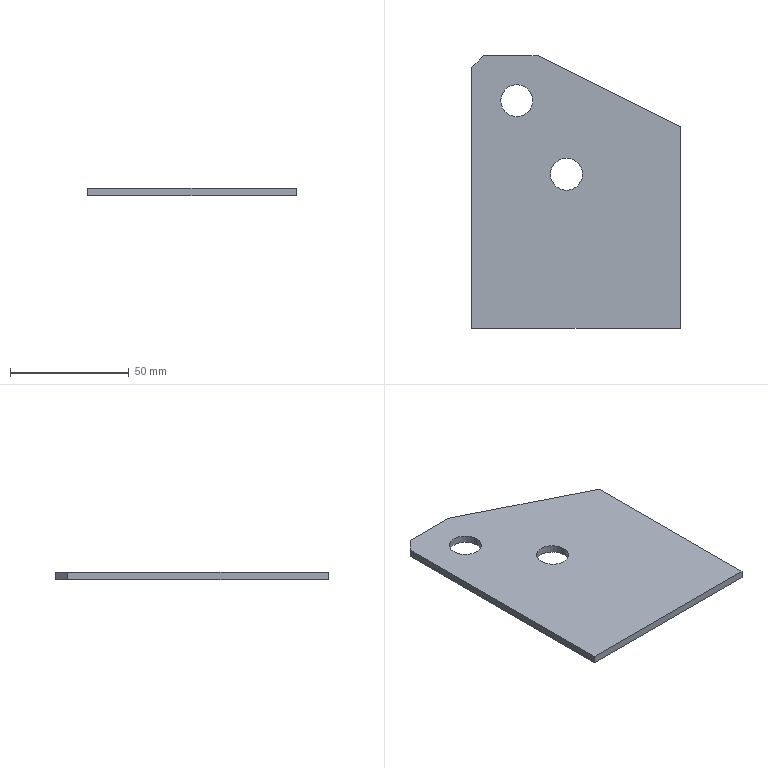Part | SolidWorks | features FlatPattern 1, SMBaseFlange 1, SheetMetal 1 | 1 solid | 12 faces | box 88 x 115 x 3.2 mm | volume 28548 mm3 | plane 8 | cylinder 4 | commonest cylinder face diameters 13.5 x4
STEP:
#1=CARTESIAN_POINT('',(17076.068,-96501.175,-3.2));
#2=VERTEX_POINT('',#1);
#3=CARTESIAN_POINT('',(17089.568,-96501.175,-3.2));
#4=VERTEX_POINT('',#3);
#5=CARTESIAN_POINT('',(17082.818,-96501.175,-3.2));
#6=DIRECTION('',(0.,0.,1.));
#7=DIRECTION('',(1.,0.,0.));
#8=AXIS2_PLACEMENT_3D('',#5,#6,#7);
#9=CIRCLE('',#8,6.75);
#10=EDGE_CURVE('',#2,#4,#9,.T.);
#11=ORIENTED_EDGE('',*,*,#10,.F.);
#12=CARTESIAN_POINT('',(17076.068,-96501.175,0.));
#13=VERTEX_POINT('',#12);
#14=CARTESIAN_POINT('',(17076.068,-96501.175,-3.2));
#15=DIRECTION('',(0.,0.,1.));
#16=VECTOR('',#15,1000.);
#17=LINE('',#14,#16);
#18=EDGE_CURVE('',#2,#13,#17,.T.);
#19=ORIENTED_EDGE('',*,*,#18,.T.);
#20=CARTESIAN_POINT('',(17089.568,-96501.175,0.));
#21=VERTEX_POINT('',#20);
#22=CARTESIAN_POINT('',(17082.818,-96501.175,0.));
#23=DIRECTION('',(0.,0.,1.));
#24=DIRECTION('',(1.,0.,0.));
#25=AXIS2_PLACEMENT_3D('',#22,#23,#24);
#26=CIRCLE('',#25,6.75);
#27=EDGE_CURVE('',#13,#21,#26,.T.);
#28=ORIENTED_EDGE('',*,*,#27,.T.);
#29=CARTESIAN_POINT('',(17089.568,-96501.175,-3.2));
#30=DIRECTION('',(0.,0.,1.));
#31=VECTOR('',#30,1000.);
#32=LINE('',#29,#31);
#33=EDGE_CURVE('',#4,#21,#32,.T.);
#34=ORIENTED_EDGE('',*,*,#33,.F.);
#35=EDGE_LOOP('',(#11,#19,#28,#34));
#36=FACE_OUTER_BOUND('',#35,.T.);
#37=CARTESIAN_POINT('',(17082.818,-96501.175,-3.2));
#38=DIRECTION('',(0.,0.,1.));
#39=DIRECTION('',(1.,0.,0.));
#40=AXIS2_PLACEMENT_3D('',#37,#38,#39);
#41=CYLINDRICAL_SURFACE('',#40,6.75);
#42=ADVANCED_FACE('',(#36),#41,.F.);
#43=CARTESIAN_POINT('',(17097.068,-96532.175,-3.2));
#44=VERTEX_POINT('',#43);
#45=CARTESIAN_POINT('',(17110.568,-96532.175,-3.2));
#46=VERTEX_POINT('',#45);
#47=CARTESIAN_POINT('',(17103.818,-96532.175,-3.2));
#48=DIRECTION('',(0.,0.,1.));
#49=DIRECTION('',(1.,0.,0.));
#50=AXIS2_PLACEMENT_3D('',#47,#48,#49);
#51=CIRCLE('',#50,6.75);
#52=EDGE_CURVE('',#44,#46,#51,.T.);
#53=ORIENTED_EDGE('',*,*,#52,.F.);
#54=CARTESIAN_POINT('',(17097.068,-96532.175,0.));
#55=VERTEX_POINT('',#54);
#56=CARTESIAN_POINT('',(17097.068,-96532.175,-3.2));
#57=DIRECTION('',(0.,0.,1.));
#58=VECTOR('',#57,1000.);
#59=LINE('',#56,#58);
#60=EDGE_CURVE('',#44,#55,#59,.T.);
#61=ORIENTED_EDGE('',*,*,#60,.T.);
#62=CARTESIAN_POINT('',(17110.568,-96532.175,0.));
#63=VERTEX_POINT('',#62);
#64=CARTESIAN_POINT('',(17103.818,-96532.175,0.));
#65=DIRECTION('',(0.,0.,1.));
#66=DIRECTION('',(1.,0.,0.));
#67=AXIS2_PLACEMENT_3D('',#64,#65,#66);
#68=CIRCLE('',#67,6.75);
#69=EDGE_CURVE('',#55,#63,#68,.T.);
#70=ORIENTED_EDGE('',*,*,#69,.T.);
#71=CARTESIAN_POINT('',(17110.568,-96532.175,-3.2));
#72=DIRECTION('',(0.,0.,1.));
#73=VECTOR('',#72,1000.);
#74=LINE('',#71,#73);
#75=EDGE_CURVE('',#46,#63,#74,.T.);
#76=ORIENTED_EDGE('',*,*,#75,.F.);
#77=EDGE_LOOP('',(#53,#61,#70,#76));
#78=FACE_OUTER_BOUND('',#77,.T.);
#79=CARTESIAN_POINT('',(17103.818,-96532.175,-3.2));
#80=DIRECTION('',(0.,0.,1.));
#81=DIRECTION('',(1.,0.,0.));
#82=AXIS2_PLACEMENT_3D('',#79,#80,#81);
#83=CYLINDRICAL_SURFACE('',#82,6.75);
#84=ADVANCED_FACE('',(#78),#83,.F.);
#85=CARTESIAN_POINT('',(17063.818,-96597.175,0.));
#86=VERTEX_POINT('',#85);
#87=CARTESIAN_POINT('',(17151.818,-96597.175,0.));
#88=VERTEX_POINT('',#87);
#89=CARTESIAN_POINT('',(17151.818,-96597.175,0.));
#90=DIRECTION('',(1.,0.,0.));
#91=VECTOR('',#90,1000.);
#92=LINE('',#89,#91);
#93=EDGE_CURVE('',#86,#88,#92,.T.);
#94=ORIENTED_EDGE('',*,*,#93,.F.);
#95=CARTESIAN_POINT('',(17063.818,-96597.175,-3.2));
#96=VERTEX_POINT('',#95);
#97=CARTESIAN_POINT('',(17063.818,-96597.175,-3.2));
#98=DIRECTION('',(0.,0.,1.));
#99=VECTOR('',#98,1000.);
#100=LINE('',#97,#99);
#101=EDGE_CURVE('',#96,#86,#100,.T.);
#102=ORIENTED_EDGE('',*,*,#101,.F.);
#103=CARTESIAN_POINT('',(17151.818,-96597.175,-3.2));
#104=VERTEX_POINT('',#103);
#105=CARTESIAN_POINT('',(17151.818,-96597.175,-3.2));
#106=DIRECTION('',(1.,0.,0.));
#107=VECTOR('',#106,1000.);
#108=LINE('',#105,#107);
#109=EDGE_CURVE('',#96,#104,#108,.T.);
#110=ORIENTED_EDGE('',*,*,#109,.T.);
#111=CARTESIAN_POINT('',(17151.818,-96597.175,-3.2));
#112=DIRECTION('',(0.,0.,1.));
#113=VECTOR('',#112,1000.);
#114=LINE('',#111,#113);
#115=EDGE_CURVE('',#104,#88,#114,.T.);
#116=ORIENTED_EDGE('',*,*,#115,.T.);
#117=EDGE_LOOP('',(#94,#102,#110,#116));
#118=FACE_OUTER_BOUND('',#117,.T.);
#119=CARTESIAN_POINT('',(17151.818,-96597.175,-3.2));
#120=DIRECTION('',(0.,-1.,0.));
#121=DIRECTION('',(0.,0.,-1.));
#122=AXIS2_PLACEMENT_3D('',#119,#120,#121);
#123=PLANE('',#122);
#124=ADVANCED_FACE('',(#118),#123,.T.);
#125=CARTESIAN_POINT('',(17063.818,-96487.175,0.));
#126=VERTEX_POINT('',#125);
#127=CARTESIAN_POINT('',(17063.818,-96597.175,0.));
#128=DIRECTION('',(0.,-1.,0.));
#129=VECTOR('',#128,1000.);
#130=LINE('',#127,#129);
#131=EDGE_CURVE('',#126,#86,#130,.T.);
#132=ORIENTED_EDGE('',*,*,#131,.F.);
#133=CARTESIAN_POINT('',(17063.818,-96487.175,-3.2));
#134=VERTEX_POINT('',#133);
#135=CARTESIAN_POINT('',(17063.818,-96487.175,-3.2));
#136=DIRECTION('',(0.,0.,1.));
#137=VECTOR('',#136,1000.);
#138=LINE('',#135,#137);
#139=EDGE_CURVE('',#134,#126,#138,.T.);
#140=ORIENTED_EDGE('',*,*,#139,.F.);
#141=CARTESIAN_POINT('',(17063.818,-96584.675,-3.2));
#142=DIRECTION('',(0.,-1.,0.));
#143=VECTOR('',#142,1000.);
#144=LINE('',#141,#143);
#145=EDGE_CURVE('',#134,#96,#144,.T.);
#146=ORIENTED_EDGE('',*,*,#145,.T.);
#147=ORIENTED_EDGE('',*,*,#101,.T.);
#148=EDGE_LOOP('',(#132,#140,#146,#147));
#149=FACE_OUTER_BOUND('',#148,.T.);
#150=CARTESIAN_POINT('',(17063.818,-96597.175,-3.2));
#151=DIRECTION('',(-1.,0.,0.));
#152=DIRECTION('',(0.,0.,1.));
#153=AXIS2_PLACEMENT_3D('',#150,#151,#152);
#154=PLANE('',#153);
#155=ADVANCED_FACE('',(#149),#154,.T.);
#156=CARTESIAN_POINT('',(17068.818,-96482.175,0.));
#157=VERTEX_POINT('',#156);
#158=CARTESIAN_POINT('',(17068.818,-96482.175,0.));
#159=DIRECTION('',(-0.7071,-0.7071,0.));
#160=VECTOR('',#159,1000.);
#161=LINE('',#158,#160);
#162=EDGE_CURVE('',#157,#126,#161,.T.);
#163=ORIENTED_EDGE('',*,*,#162,.F.);
#164=CARTESIAN_POINT('',(17068.818,-96482.175,-3.2));
#165=VERTEX_POINT('',#164);
#166=CARTESIAN_POINT('',(17068.818,-96482.175,-3.2));
#167=DIRECTION('',(0.,0.,1.));
#168=VECTOR('',#167,1000.);
#169=LINE('',#166,#168);
#170=EDGE_CURVE('',#165,#157,#169,.T.);
#171=ORIENTED_EDGE('',*,*,#170,.F.);
#172=CARTESIAN_POINT('',(17068.818,-96482.175,-3.2));
#173=DIRECTION('',(-0.7071,-0.7071,0.));
#174=VECTOR('',#173,1000.);
#175=LINE('',#172,#174);
#176=EDGE_CURVE('',#165,#134,#175,.T.);
#177=ORIENTED_EDGE('',*,*,#176,.T.);
#178=ORIENTED_EDGE('',*,*,#139,.T.);
#179=EDGE_LOOP('',(#163,#171,#177,#178));
#180=FACE_OUTER_BOUND('',#179,.T.);
#181=CARTESIAN_POINT('',(17068.818,-96482.175,-3.2));
#182=DIRECTION('',(-0.7071,0.7071,0.));
#183=DIRECTION('',(-0.7071,-0.7071,0.));
#184=AXIS2_PLACEMENT_3D('',#181,#182,#183);
#185=PLANE('',#184);
#186=ADVANCED_FACE('',(#180),#185,.T.);
#187=CARTESIAN_POINT('',(17091.818,-96482.175,0.));
#188=VERTEX_POINT('',#187);
#189=CARTESIAN_POINT('',(17068.818,-96482.175,0.));
#190=DIRECTION('',(-1.,0.,0.));
#191=VECTOR('',#190,1000.);
#192=LINE('',#189,#191);
#193=EDGE_CURVE('',#188,#157,#192,.T.);
#194=ORIENTED_EDGE('',*,*,#193,.F.);
#195=CARTESIAN_POINT('',(17091.818,-96482.175,-3.2));
#196=VERTEX_POINT('',#195);
#197=CARTESIAN_POINT('',(17091.818,-96482.175,-3.2));
#198=DIRECTION('',(0.,0.,1.));
#199=VECTOR('',#198,1000.);
#200=LINE('',#197,#199);
#201=EDGE_CURVE('',#196,#188,#200,.T.);
#202=ORIENTED_EDGE('',*,*,#201,.F.);
#203=CARTESIAN_POINT('',(17068.818,-96482.175,-3.2));
#204=DIRECTION('',(-1.,0.,0.));
#205=VECTOR('',#204,1000.);
#206=LINE('',#203,#205);
#207=EDGE_CURVE('',#196,#165,#206,.T.);
#208=ORIENTED_EDGE('',*,*,#207,.T.);
#209=ORIENTED_EDGE('',*,*,#170,.T.);
#210=EDGE_LOOP('',(#194,#202,#208,#209));
#211=FACE_OUTER_BOUND('',#210,.T.);
#212=CARTESIAN_POINT('',(17068.818,-96482.175,-3.2));
#213=DIRECTION('',(0.,1.,0.));
#214=DIRECTION('',(0.,0.,1.));
#215=AXIS2_PLACEMENT_3D('',#212,#213,#214);
#216=PLANE('',#215);
#217=ADVANCED_FACE('',(#211),#216,.T.);
#218=CARTESIAN_POINT('',(17151.818,-96512.175,0.));
#219=VERTEX_POINT('',#218);
#220=CARTESIAN_POINT('',(17091.818,-96482.175,0.));
#221=DIRECTION('',(-0.8944,0.4472,0.));
#222=VECTOR('',#221,1000.);
#223=LINE('',#220,#222);
#224=EDGE_CURVE('',#219,#188,#223,.T.);
#225=ORIENTED_EDGE('',*,*,#224,.F.);
#226=CARTESIAN_POINT('',(17151.818,-96512.175,-3.2));
#227=VERTEX_POINT('',#226);
#228=CARTESIAN_POINT('',(17151.818,-96512.175,-3.2));
#229=DIRECTION('',(0.,0.,1.));
#230=VECTOR('',#229,1000.);
#231=LINE('',#228,#230);
#232=EDGE_CURVE('',#227,#219,#231,.T.);
#233=ORIENTED_EDGE('',*,*,#232,.F.);
#234=CARTESIAN_POINT('',(17091.818,-96482.175,-3.2));
#235=DIRECTION('',(-0.8944,0.4472,0.));
#236=VECTOR('',#235,1000.);
#237=LINE('',#234,#236);
#238=EDGE_CURVE('',#227,#196,#237,.T.);
#239=ORIENTED_EDGE('',*,*,#238,.T.);
#240=ORIENTED_EDGE('',*,*,#201,.T.);
#241=EDGE_LOOP('',(#225,#233,#239,#240));
#242=FACE_OUTER_BOUND('',#241,.T.);
#243=CARTESIAN_POINT('',(17091.818,-96482.175,-3.2));
#244=DIRECTION('',(0.4472,0.8944,0.));
#245=DIRECTION('',(-0.8944,0.4472,0.));
#246=AXIS2_PLACEMENT_3D('',#243,#244,#245);
#247=PLANE('',#246);
#248=ADVANCED_FACE('',(#242),#247,.T.);
#249=CARTESIAN_POINT('',(17151.818,-96512.175,0.));
#250=DIRECTION('',(0.,1.,0.));
#251=VECTOR('',#250,1000.);
#252=LINE('',#249,#251);
#253=EDGE_CURVE('',#88,#219,#252,.T.);
#254=ORIENTED_EDGE('',*,*,#253,.F.);
#255=ORIENTED_EDGE('',*,*,#115,.F.);
#256=CARTESIAN_POINT('',(17151.818,-96584.675,-3.2));
#257=DIRECTION('',(0.,1.,0.));
#258=VECTOR('',#257,1000.);
#259=LINE('',#256,#258);
#260=EDGE_CURVE('',#104,#227,#259,.T.);
#261=ORIENTED_EDGE('',*,*,#260,.T.);
#262=ORIENTED_EDGE('',*,*,#232,.T.);
#263=EDGE_LOOP('',(#254,#255,#261,#262));
#264=FACE_OUTER_BOUND('',#263,.T.);
#265=CARTESIAN_POINT('',(17151.818,-96512.175,-3.2));
#266=DIRECTION('',(1.,0.,0.));
#267=DIRECTION('',(0.,0.,-1.));
#268=AXIS2_PLACEMENT_3D('',#265,#266,#267);
#269=PLANE('',#268);
#270=ADVANCED_FACE('',(#264),#269,.T.);
#271=CARTESIAN_POINT('',(17082.818,-96501.175,-3.2));
#272=DIRECTION('',(0.,0.,1.));
#273=DIRECTION('',(1.,0.,0.));
#274=AXIS2_PLACEMENT_3D('',#271,#272,#273);
#275=CIRCLE('',#274,6.75);
#276=EDGE_CURVE('',#4,#2,#275,.T.);
#277=ORIENTED_EDGE('',*,*,#276,.T.);
#278=ORIENTED_EDGE('',*,*,#10,.T.);
#279=EDGE_LOOP('',(#277,#278));
#280=FACE_BOUND('',#279,.T.);
#281=CARTESIAN_POINT('',(17103.818,-96532.175,-3.2));
#282=DIRECTION('',(0.,0.,1.));
#283=DIRECTION('',(1.,0.,0.));
#284=AXIS2_PLACEMENT_3D('',#281,#282,#283);
#285=CIRCLE('',#284,6.75);
#286=EDGE_CURVE('',#46,#44,#285,.T.);
#287=ORIENTED_EDGE('',*,*,#286,.T.);
#288=ORIENTED_EDGE('',*,*,#52,.T.);
#289=EDGE_LOOP('',(#287,#288));
#290=FACE_BOUND('',#289,.T.);
#291=ORIENTED_EDGE('',*,*,#109,.F.);
#292=ORIENTED_EDGE('',*,*,#145,.F.);
#293=ORIENTED_EDGE('',*,*,#176,.F.);
#294=ORIENTED_EDGE('',*,*,#207,.F.);
#295=ORIENTED_EDGE('',*,*,#238,.F.);
#296=ORIENTED_EDGE('',*,*,#260,.F.);
#297=EDGE_LOOP('',(#291,#292,#293,#294,#295,#296));
#298=FACE_OUTER_BOUND('',#297,.T.);
#299=CARTESIAN_POINT('',(0.,0.,-3.2));
#300=DIRECTION('',(0.,0.,-1.));
#301=DIRECTION('',(-1.,0.,0.));
#302=AXIS2_PLACEMENT_3D('',#299,#300,#301);
#303=PLANE('',#302);
#304=ADVANCED_FACE('',(#280,#290,#298),#303,.T.);
#305=CARTESIAN_POINT('',(17082.818,-96501.175,0.));
#306=DIRECTION('',(0.,0.,1.));
#307=DIRECTION('',(1.,0.,0.));
#308=AXIS2_PLACEMENT_3D('',#305,#306,#307);
#309=CIRCLE('',#308,6.75);
#310=EDGE_CURVE('',#21,#13,#309,.T.);
#311=ORIENTED_EDGE('',*,*,#310,.F.);
#312=ORIENTED_EDGE('',*,*,#27,.F.);
#313=EDGE_LOOP('',(#311,#312));
#314=FACE_BOUND('',#313,.T.);
#315=CARTESIAN_POINT('',(17103.818,-96532.175,0.));
#316=DIRECTION('',(0.,0.,1.));
#317=DIRECTION('',(1.,0.,0.));
#318=AXIS2_PLACEMENT_3D('',#315,#316,#317);
#319=CIRCLE('',#318,6.75);
#320=EDGE_CURVE('',#63,#55,#319,.T.);
#321=ORIENTED_EDGE('',*,*,#320,.F.);
#322=ORIENTED_EDGE('',*,*,#69,.F.);
#323=EDGE_LOOP('',(#321,#322));
#324=FACE_BOUND('',#323,.T.);
#325=ORIENTED_EDGE('',*,*,#93,.T.);
#326=ORIENTED_EDGE('',*,*,#253,.T.);
#327=ORIENTED_EDGE('',*,*,#224,.T.);
#328=ORIENTED_EDGE('',*,*,#193,.T.);
#329=ORIENTED_EDGE('',*,*,#162,.T.);
#330=ORIENTED_EDGE('',*,*,#131,.T.);
#331=EDGE_LOOP('',(#325,#326,#327,#328,#329,#330));
#332=FACE_OUTER_BOUND('',#331,.T.);
#333=CARTESIAN_POINT('',(0.,0.,0.));
#334=DIRECTION('',(0.,0.,-1.));
#335=DIRECTION('',(-1.,0.,0.));
#336=AXIS2_PLACEMENT_3D('',#333,#334,#335);
#337=PLANE('',#336);
#338=ADVANCED_FACE('',(#314,#324,#332),#337,.F.);
#339=ORIENTED_EDGE('',*,*,#60,.F.);
#340=ORIENTED_EDGE('',*,*,#286,.F.);
#341=ORIENTED_EDGE('',*,*,#75,.T.);
#342=ORIENTED_EDGE('',*,*,#320,.T.);
#343=EDGE_LOOP('',(#339,#340,#341,#342));
#344=FACE_OUTER_BOUND('',#343,.T.);
#345=CARTESIAN_POINT('',(17103.818,-96532.175,-3.2));
#346=DIRECTION('',(0.,0.,1.));
#347=DIRECTION('',(1.,0.,0.));
#348=AXIS2_PLACEMENT_3D('',#345,#346,#347);
#349=CYLINDRICAL_SURFACE('',#348,6.75);
#350=ADVANCED_FACE('',(#344),#349,.F.);
#351=ORIENTED_EDGE('',*,*,#18,.F.);
#352=ORIENTED_EDGE('',*,*,#276,.F.);
#353=ORIENTED_EDGE('',*,*,#33,.T.);
#354=ORIENTED_EDGE('',*,*,#310,.T.);
#355=EDGE_LOOP('',(#351,#352,#353,#354));
#356=FACE_OUTER_BOUND('',#355,.T.);
#357=CARTESIAN_POINT('',(17082.818,-96501.175,-3.2));
#358=DIRECTION('',(0.,0.,1.));
#359=DIRECTION('',(1.,0.,0.));
#360=AXIS2_PLACEMENT_3D('',#357,#358,#359);
#361=CYLINDRICAL_SURFACE('',#360,6.75);
#362=ADVANCED_FACE('',(#356),#361,.F.);
#363=CLOSED_SHELL('',(#42,#84,#124,#155,#186,#217,#248,#270,#304,#338,#350,#362));
#364=MANIFOLD_SOLID_BREP('',#363);
#365=CARTESIAN_POINT('',(0.,0.,0.));
#366=DIRECTION('',(0.,0.,1.));
#367=DIRECTION('',(1.,0.,0.));
#368=AXIS2_PLACEMENT_3D('',#365,#366,#367);
#369=(LENGTH_UNIT()NAMED_UNIT(*)SI_UNIT(.MILLI.,.METRE.));
#370=UNCERTAINTY_MEASURE_WITH_UNIT(LENGTH_MEASURE(0.00001),#369,'','');
#371=(NAMED_UNIT(*)PLANE_ANGLE_UNIT()SI_UNIT($,.RADIAN.));
#372=(NAMED_UNIT(*)SI_UNIT($,.STERADIAN.)SOLID_ANGLE_UNIT());
#373=(GEOMETRIC_REPRESENTATION_CONTEXT(3)GLOBAL_UNCERTAINTY_ASSIGNED_CONTEXT((#370))GLOBAL_UNIT_ASSIGNED_CONTEXT((#369,#371,#372))REPRESENTATION_CONTEXT('',''));
#374=ADVANCED_BREP_SHAPE_REPRESENTATION('',(#364,#368),#373);